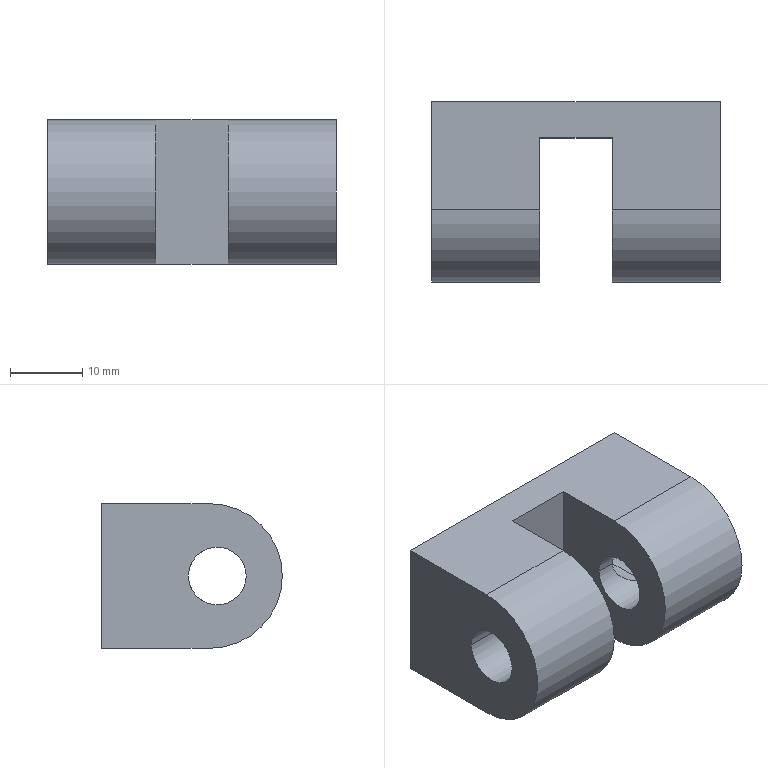Part | SolidWorks | features BaseBody 1 | 1 solid | 18 faces | box 40 x 25 x 20 mm | volume 12303 mm3 | cylinder 10 | plane 8 | commonest cylinder face diameters 6.8 x4 8 x4 20 x2
STEP:
#1=CARTESIAN_POINT('',(5.,-7.5,10.));
#2=VERTEX_POINT('',#1);
#3=CARTESIAN_POINT('',(5.,0.5,10.));
#4=VERTEX_POINT('',#3);
#5=CARTESIAN_POINT('',(5.,-3.5,10.));
#6=DIRECTION('',(1.,0.,0.));
#7=DIRECTION('',(0.,0.,-1.));
#8=AXIS2_PLACEMENT_3D('',#5,#6,#7);
#9=CIRCLE('',#8,4.);
#10=EDGE_CURVE('',#2,#4,#9,.T.);
#11=ORIENTED_EDGE('',*,*,#10,.F.);
#12=CARTESIAN_POINT('',(20.,-7.5,10.));
#13=VERTEX_POINT('',#12);
#14=CARTESIAN_POINT('',(-20.,-7.5,10.));
#15=DIRECTION('',(1.,0.,0.));
#16=VECTOR('',#15,1000.);
#17=LINE('',#14,#16);
#18=EDGE_CURVE('',#2,#13,#17,.T.);
#19=ORIENTED_EDGE('',*,*,#18,.T.);
#20=CARTESIAN_POINT('',(20.,0.5,10.));
#21=VERTEX_POINT('',#20);
#22=CARTESIAN_POINT('',(20.,-3.5,10.));
#23=DIRECTION('',(1.,0.,0.));
#24=DIRECTION('',(0.,1.,0.));
#25=AXIS2_PLACEMENT_3D('',#22,#23,#24);
#26=CIRCLE('',#25,4.);
#27=EDGE_CURVE('',#13,#21,#26,.T.);
#28=ORIENTED_EDGE('',*,*,#27,.T.);
#29=CARTESIAN_POINT('',(14.4,0.5,10.));
#30=VERTEX_POINT('',#29);
#31=CARTESIAN_POINT('',(-20.,0.5,10.));
#32=DIRECTION('',(1.,0.,0.));
#33=VECTOR('',#32,1000.);
#34=LINE('',#31,#33);
#35=EDGE_CURVE('',#30,#21,#34,.T.);
#36=ORIENTED_EDGE('',*,*,#35,.F.);
#37=CARTESIAN_POINT('',(11.,-1.393,6.6));
#38=VERTEX_POINT('',#37);
#39=CARTESIAN_POINT('',(11.,-1.393,6.6));
#40=CARTESIAN_POINT('',(11.242,-1.393,6.6));
#41=CARTESIAN_POINT('',(11.476,-1.35,6.626));
#42=CARTESIAN_POINT('',(11.927,-1.208,6.721));
#43=CARTESIAN_POINT('',(12.134,-1.113,6.788));
#44=CARTESIAN_POINT('',(12.529,-0.9021,6.956));
#45=CARTESIAN_POINT('',(12.715,-0.7863,7.057));
#46=CARTESIAN_POINT('',(13.06,-0.5558,7.287));
#47=CARTESIAN_POINT('',(13.221,-0.44,7.417));
#48=CARTESIAN_POINT('',(13.522,-0.2151,7.71));
#49=CARTESIAN_POINT('',(13.662,-0.1055,7.874));
#50=CARTESIAN_POINT('',(13.91,0.09224,8.229));
#51=CARTESIAN_POINT('',(14.019,0.1816,8.42));
#52=CARTESIAN_POINT('',(14.204,0.3341,8.838));
#53=CARTESIAN_POINT('',(14.275,0.3945,9.058));
#54=CARTESIAN_POINT('',(14.374,0.4777,9.518));
#55=CARTESIAN_POINT('',(14.4,0.5,9.759));
#56=CARTESIAN_POINT('',(14.4,0.5,10.));
#57=B_SPLINE_CURVE_WITH_KNOTS('',3,(#39,#40,#41,#42,#43,#44,#45,#46,#47,#48,#49,#50,#51,#52,#53,#54,#55,#56),.UNSPECIFIED.,.F.,.F.,(4,2,2,2,2,2,2,2,4),(0.,0.0007143,0.001429,0.002143,0.002857,0.003571,0.004286,0.005,0.005714),.UNSPECIFIED.);
#58=EDGE_CURVE('',#38,#30,#57,.T.);
#59=ORIENTED_EDGE('',*,*,#58,.F.);
#60=CARTESIAN_POINT('',(7.6,0.5,10.));
#61=VERTEX_POINT('',#60);
#62=CARTESIAN_POINT('',(7.6,0.5,10.));
#63=CARTESIAN_POINT('',(7.6,0.5,9.759));
#64=CARTESIAN_POINT('',(7.625,0.4783,9.523));
#65=CARTESIAN_POINT('',(7.723,0.396,9.064));
#66=CARTESIAN_POINT('',(7.796,0.3345,8.84));
#67=CARTESIAN_POINT('',(7.978,0.1841,8.426));
#68=CARTESIAN_POINT('',(8.088,0.09337,8.231));
#69=CARTESIAN_POINT('',(8.337,-0.1049,7.875));
#70=CARTESIAN_POINT('',(8.474,-0.2123,7.714));
#71=CARTESIAN_POINT('',(8.774,-0.4367,7.421));
#72=CARTESIAN_POINT('',(8.938,-0.5549,7.288));
#73=CARTESIAN_POINT('',(9.285,-0.786,7.057));
#74=CARTESIAN_POINT('',(9.467,-0.8998,6.957));
#75=CARTESIAN_POINT('',(9.861,-1.11,6.789));
#76=CARTESIAN_POINT('',(10.073,-1.208,6.721));
#77=CARTESIAN_POINT('',(10.519,-1.349,6.627));
#78=CARTESIAN_POINT('',(10.758,-1.393,6.6));
#79=CARTESIAN_POINT('',(11.,-1.393,6.6));
#80=B_SPLINE_CURVE_WITH_KNOTS('',3,(#62,#63,#64,#65,#66,#67,#68,#69,#70,#71,#72,#73,#74,#75,#76,#77,#78,#79),.UNSPECIFIED.,.F.,.F.,(4,2,2,2,2,2,2,2,4),(0.01715,0.01786,0.01858,0.01929,0.02001,0.02072,0.02144,0.02215,0.02287),.UNSPECIFIED.);
#81=EDGE_CURVE('',#61,#38,#80,.T.);
#82=ORIENTED_EDGE('',*,*,#81,.F.);
#83=CARTESIAN_POINT('',(-20.,0.5,10.));
#84=DIRECTION('',(1.,0.,0.));
#85=VECTOR('',#84,1000.);
#86=LINE('',#83,#85);
#87=EDGE_CURVE('',#4,#61,#86,.T.);
#88=ORIENTED_EDGE('',*,*,#87,.F.);
#89=EDGE_LOOP('',(#11,#19,#28,#36,#59,#82,#88));
#90=FACE_OUTER_BOUND('',#89,.T.);
#91=CARTESIAN_POINT('',(-20.,-3.5,10.));
#92=DIRECTION('',(1.,0.,0.));
#93=DIRECTION('',(0.,1.,0.));
#94=AXIS2_PLACEMENT_3D('',#91,#92,#93);
#95=CYLINDRICAL_SURFACE('',#94,4.);
#96=ADVANCED_FACE('',(#90),#95,.F.);
#97=CARTESIAN_POINT('',(-20.,-7.5,10.));
#98=VERTEX_POINT('',#97);
#99=CARTESIAN_POINT('',(-20.,0.5,10.));
#100=VERTEX_POINT('',#99);
#101=CARTESIAN_POINT('',(-20.,-3.5,10.));
#102=DIRECTION('',(1.,0.,0.));
#103=DIRECTION('',(0.,1.,0.));
#104=AXIS2_PLACEMENT_3D('',#101,#102,#103);
#105=CIRCLE('',#104,4.);
#106=EDGE_CURVE('',#98,#100,#105,.T.);
#107=ORIENTED_EDGE('',*,*,#106,.F.);
#108=CARTESIAN_POINT('',(-5.,-7.5,10.));
#109=VERTEX_POINT('',#108);
#110=CARTESIAN_POINT('',(-20.,-7.5,10.));
#111=DIRECTION('',(1.,0.,0.));
#112=VECTOR('',#111,1000.);
#113=LINE('',#110,#112);
#114=EDGE_CURVE('',#98,#109,#113,.T.);
#115=ORIENTED_EDGE('',*,*,#114,.T.);
#116=CARTESIAN_POINT('',(-5.,0.5,10.));
#117=VERTEX_POINT('',#116);
#118=CARTESIAN_POINT('',(-5.,-3.5,10.));
#119=DIRECTION('',(-1.,0.,0.));
#120=DIRECTION('',(0.,0.,1.));
#121=AXIS2_PLACEMENT_3D('',#118,#119,#120);
#122=CIRCLE('',#121,4.);
#123=EDGE_CURVE('',#117,#109,#122,.T.);
#124=ORIENTED_EDGE('',*,*,#123,.F.);
#125=CARTESIAN_POINT('',(-7.6,0.5,10.));
#126=VERTEX_POINT('',#125);
#127=CARTESIAN_POINT('',(-20.,0.5,10.));
#128=DIRECTION('',(1.,0.,0.));
#129=VECTOR('',#128,1000.);
#130=LINE('',#127,#129);
#131=EDGE_CURVE('',#126,#117,#130,.T.);
#132=ORIENTED_EDGE('',*,*,#131,.F.);
#133=CARTESIAN_POINT('',(-11.,-1.393,6.6));
#134=VERTEX_POINT('',#133);
#135=CARTESIAN_POINT('',(-11.,-1.393,6.6));
#136=CARTESIAN_POINT('',(-10.758,-1.393,6.6));
#137=CARTESIAN_POINT('',(-10.524,-1.35,6.626));
#138=CARTESIAN_POINT('',(-10.073,-1.208,6.721));
#139=CARTESIAN_POINT('',(-9.866,-1.113,6.788));
#140=CARTESIAN_POINT('',(-9.471,-0.9021,6.956));
#141=CARTESIAN_POINT('',(-9.285,-0.7863,7.057));
#142=CARTESIAN_POINT('',(-8.94,-0.5558,7.287));
#143=CARTESIAN_POINT('',(-8.779,-0.44,7.417));
#144=CARTESIAN_POINT('',(-8.478,-0.2151,7.71));
#145=CARTESIAN_POINT('',(-8.338,-0.1055,7.874));
#146=CARTESIAN_POINT('',(-8.09,0.09224,8.229));
#147=CARTESIAN_POINT('',(-7.981,0.1816,8.42));
#148=CARTESIAN_POINT('',(-7.796,0.3341,8.838));
#149=CARTESIAN_POINT('',(-7.725,0.3945,9.058));
#150=CARTESIAN_POINT('',(-7.626,0.4777,9.518));
#151=CARTESIAN_POINT('',(-7.6,0.5,9.759));
#152=CARTESIAN_POINT('',(-7.6,0.5,10.));
#153=B_SPLINE_CURVE_WITH_KNOTS('',3,(#135,#136,#137,#138,#139,#140,#141,#142,#143,#144,#145,#146,#147,#148,#149,#150,#151,#152),.UNSPECIFIED.,.F.,.F.,(4,2,2,2,2,2,2,2,4),(0.,0.0007143,0.001429,0.002143,0.002857,0.003571,0.004286,0.005,0.005714),.UNSPECIFIED.);
#154=EDGE_CURVE('',#134,#126,#153,.T.);
#155=ORIENTED_EDGE('',*,*,#154,.F.);
#156=CARTESIAN_POINT('',(-14.4,0.5,10.));
#157=VERTEX_POINT('',#156);
#158=CARTESIAN_POINT('',(-14.4,0.5,10.));
#159=CARTESIAN_POINT('',(-14.4,0.5,9.759));
#160=CARTESIAN_POINT('',(-14.375,0.4783,9.523));
#161=CARTESIAN_POINT('',(-14.277,0.396,9.064));
#162=CARTESIAN_POINT('',(-14.204,0.3345,8.84));
#163=CARTESIAN_POINT('',(-14.022,0.1841,8.426));
#164=CARTESIAN_POINT('',(-13.912,0.09337,8.231));
#165=CARTESIAN_POINT('',(-13.663,-0.1049,7.875));
#166=CARTESIAN_POINT('',(-13.526,-0.2123,7.714));
#167=CARTESIAN_POINT('',(-13.226,-0.4367,7.421));
#168=CARTESIAN_POINT('',(-13.062,-0.5549,7.288));
#169=CARTESIAN_POINT('',(-12.715,-0.786,7.057));
#170=CARTESIAN_POINT('',(-12.533,-0.8998,6.957));
#171=CARTESIAN_POINT('',(-12.139,-1.11,6.789));
#172=CARTESIAN_POINT('',(-11.927,-1.208,6.721));
#173=CARTESIAN_POINT('',(-11.481,-1.349,6.627));
#174=CARTESIAN_POINT('',(-11.242,-1.393,6.6));
#175=CARTESIAN_POINT('',(-11.,-1.393,6.6));
#176=B_SPLINE_CURVE_WITH_KNOTS('',3,(#158,#159,#160,#161,#162,#163,#164,#165,#166,#167,#168,#169,#170,#171,#172,#173,#174,#175),.UNSPECIFIED.,.F.,.F.,(4,2,2,2,2,2,2,2,4),(0.01715,0.01786,0.01858,0.01929,0.02001,0.02072,0.02144,0.02215,0.02287),.UNSPECIFIED.);
#177=EDGE_CURVE('',#157,#134,#176,.T.);
#178=ORIENTED_EDGE('',*,*,#177,.F.);
#179=CARTESIAN_POINT('',(-20.,0.5,10.));
#180=DIRECTION('',(1.,0.,0.));
#181=VECTOR('',#180,1000.);
#182=LINE('',#179,#181);
#183=EDGE_CURVE('',#100,#157,#182,.T.);
#184=ORIENTED_EDGE('',*,*,#183,.F.);
#185=EDGE_LOOP('',(#107,#115,#124,#132,#155,#178,#184));
#186=FACE_OUTER_BOUND('',#185,.T.);
#187=CARTESIAN_POINT('',(-20.,-3.5,10.));
#188=DIRECTION('',(1.,0.,0.));
#189=DIRECTION('',(0.,1.,0.));
#190=AXIS2_PLACEMENT_3D('',#187,#188,#189);
#191=CYLINDRICAL_SURFACE('',#190,4.);
#192=ADVANCED_FACE('',(#186),#191,.F.);
#193=CARTESIAN_POINT('',(-11.,-1.393,13.4));
#194=VERTEX_POINT('',#193);
#195=CARTESIAN_POINT('',(-11.,-1.393,13.4));
#196=CARTESIAN_POINT('',(-11.242,-1.393,13.4));
#197=CARTESIAN_POINT('',(-11.476,-1.35,13.374));
#198=CARTESIAN_POINT('',(-11.927,-1.208,13.279));
#199=CARTESIAN_POINT('',(-12.134,-1.113,13.212));
#200=CARTESIAN_POINT('',(-12.529,-0.9021,13.044));
#201=CARTESIAN_POINT('',(-12.715,-0.7863,12.943));
#202=CARTESIAN_POINT('',(-13.06,-0.5558,12.713));
#203=CARTESIAN_POINT('',(-13.221,-0.44,12.583));
#204=CARTESIAN_POINT('',(-13.522,-0.2151,12.29));
#205=CARTESIAN_POINT('',(-13.662,-0.1055,12.126));
#206=CARTESIAN_POINT('',(-13.91,0.09224,11.771));
#207=CARTESIAN_POINT('',(-14.019,0.1816,11.58));
#208=CARTESIAN_POINT('',(-14.204,0.3341,11.162));
#209=CARTESIAN_POINT('',(-14.275,0.3945,10.942));
#210=CARTESIAN_POINT('',(-14.374,0.4777,10.482));
#211=CARTESIAN_POINT('',(-14.4,0.5,10.241));
#212=CARTESIAN_POINT('',(-14.4,0.5,10.));
#213=B_SPLINE_CURVE_WITH_KNOTS('',3,(#195,#196,#197,#198,#199,#200,#201,#202,#203,#204,#205,#206,#207,#208,#209,#210,#211,#212),.UNSPECIFIED.,.F.,.F.,(4,2,2,2,2,2,2,2,4),(0.01143,0.01214,0.01286,0.01357,0.01429,0.015,0.01572,0.01643,0.01715),.UNSPECIFIED.);
#214=EDGE_CURVE('',#194,#157,#213,.T.);
#215=ORIENTED_EDGE('',*,*,#214,.T.);
#216=ORIENTED_EDGE('',*,*,#177,.T.);
#217=CARTESIAN_POINT('',(-11.,12.5,6.6));
#218=VERTEX_POINT('',#217);
#219=CARTESIAN_POINT('',(-11.,12.5,6.6));
#220=DIRECTION('',(0.,1.,0.));
#221=VECTOR('',#220,1000.);
#222=LINE('',#219,#221);
#223=EDGE_CURVE('',#134,#218,#222,.T.);
#224=ORIENTED_EDGE('',*,*,#223,.T.);
#225=CARTESIAN_POINT('',(-11.,12.5,13.4));
#226=VERTEX_POINT('',#225);
#227=CARTESIAN_POINT('',(-11.,12.5,10.));
#228=DIRECTION('',(0.,1.,0.));
#229=DIRECTION('',(0.,0.,1.));
#230=AXIS2_PLACEMENT_3D('',#227,#228,#229);
#231=CIRCLE('',#230,3.4);
#232=EDGE_CURVE('',#218,#226,#231,.T.);
#233=ORIENTED_EDGE('',*,*,#232,.T.);
#234=CARTESIAN_POINT('',(-11.,12.5,13.4));
#235=DIRECTION('',(0.,1.,0.));
#236=VECTOR('',#235,1000.);
#237=LINE('',#234,#236);
#238=EDGE_CURVE('',#194,#226,#237,.T.);
#239=ORIENTED_EDGE('',*,*,#238,.F.);
#240=EDGE_LOOP('',(#215,#216,#224,#233,#239));
#241=FACE_OUTER_BOUND('',#240,.T.);
#242=CARTESIAN_POINT('',(-11.,12.5,10.));
#243=DIRECTION('',(0.,1.,0.));
#244=DIRECTION('',(0.,0.,1.));
#245=AXIS2_PLACEMENT_3D('',#242,#243,#244);
#246=CYLINDRICAL_SURFACE('',#245,3.4);
#247=ADVANCED_FACE('',(#241),#246,.F.);
#248=CARTESIAN_POINT('',(11.,-1.393,13.4));
#249=VERTEX_POINT('',#248);
#250=CARTESIAN_POINT('',(11.,-1.393,13.4));
#251=CARTESIAN_POINT('',(10.758,-1.393,13.4));
#252=CARTESIAN_POINT('',(10.524,-1.35,13.374));
#253=CARTESIAN_POINT('',(10.073,-1.208,13.279));
#254=CARTESIAN_POINT('',(9.866,-1.113,13.212));
#255=CARTESIAN_POINT('',(9.471,-0.9021,13.044));
#256=CARTESIAN_POINT('',(9.285,-0.7863,12.943));
#257=CARTESIAN_POINT('',(8.94,-0.5558,12.713));
#258=CARTESIAN_POINT('',(8.779,-0.44,12.583));
#259=CARTESIAN_POINT('',(8.478,-0.2151,12.29));
#260=CARTESIAN_POINT('',(8.338,-0.1055,12.126));
#261=CARTESIAN_POINT('',(8.09,0.09224,11.771));
#262=CARTESIAN_POINT('',(7.981,0.1816,11.58));
#263=CARTESIAN_POINT('',(7.796,0.3341,11.162));
#264=CARTESIAN_POINT('',(7.725,0.3945,10.942));
#265=CARTESIAN_POINT('',(7.626,0.4777,10.482));
#266=CARTESIAN_POINT('',(7.6,0.5,10.241));
#267=CARTESIAN_POINT('',(7.6,0.5,10.));
#268=B_SPLINE_CURVE_WITH_KNOTS('',3,(#250,#251,#252,#253,#254,#255,#256,#257,#258,#259,#260,#261,#262,#263,#264,#265,#266,#267),.UNSPECIFIED.,.F.,.F.,(4,2,2,2,2,2,2,2,4),(0.01143,0.01214,0.01286,0.01357,0.01429,0.015,0.01572,0.01643,0.01715),.UNSPECIFIED.);
#269=EDGE_CURVE('',#249,#61,#268,.T.);
#270=ORIENTED_EDGE('',*,*,#269,.T.);
#271=ORIENTED_EDGE('',*,*,#81,.T.);
#272=CARTESIAN_POINT('',(11.,12.5,6.6));
#273=VERTEX_POINT('',#272);
#274=CARTESIAN_POINT('',(11.,12.5,6.6));
#275=DIRECTION('',(0.,1.,0.));
#276=VECTOR('',#275,1000.);
#277=LINE('',#274,#276);
#278=EDGE_CURVE('',#38,#273,#277,.T.);
#279=ORIENTED_EDGE('',*,*,#278,.T.);
#280=CARTESIAN_POINT('',(11.,12.5,13.4));
#281=VERTEX_POINT('',#280);
#282=CARTESIAN_POINT('',(11.,12.5,10.));
#283=DIRECTION('',(0.,1.,0.));
#284=DIRECTION('',(0.,0.,1.));
#285=AXIS2_PLACEMENT_3D('',#282,#283,#284);
#286=CIRCLE('',#285,3.4);
#287=EDGE_CURVE('',#273,#281,#286,.T.);
#288=ORIENTED_EDGE('',*,*,#287,.T.);
#289=CARTESIAN_POINT('',(11.,12.5,13.4));
#290=DIRECTION('',(0.,1.,0.));
#291=VECTOR('',#290,1000.);
#292=LINE('',#289,#291);
#293=EDGE_CURVE('',#249,#281,#292,.T.);
#294=ORIENTED_EDGE('',*,*,#293,.F.);
#295=EDGE_LOOP('',(#270,#271,#279,#288,#294));
#296=FACE_OUTER_BOUND('',#295,.T.);
#297=CARTESIAN_POINT('',(11.,12.5,10.));
#298=DIRECTION('',(0.,1.,0.));
#299=DIRECTION('',(0.,0.,1.));
#300=AXIS2_PLACEMENT_3D('',#297,#298,#299);
#301=CYLINDRICAL_SURFACE('',#300,3.4);
#302=ADVANCED_FACE('',(#296),#301,.F.);
#303=CARTESIAN_POINT('',(20.,-2.5,0.));
#304=VERTEX_POINT('',#303);
#305=CARTESIAN_POINT('',(5.,-2.5,0.));
#306=VERTEX_POINT('',#305);
#307=CARTESIAN_POINT('',(0.,-2.5,0.));
#308=DIRECTION('',(-1.,0.,0.));
#309=VECTOR('',#308,1000.);
#310=LINE('',#307,#309);
#311=EDGE_CURVE('',#304,#306,#310,.T.);
#312=ORIENTED_EDGE('',*,*,#311,.F.);
#313=CARTESIAN_POINT('',(20.,-2.5,20.));
#314=VERTEX_POINT('',#313);
#315=CARTESIAN_POINT('',(20.,-2.5,10.));
#316=DIRECTION('',(1.,0.,0.));
#317=DIRECTION('',(0.,-1.,0.));
#318=AXIS2_PLACEMENT_3D('',#315,#316,#317);
#319=CIRCLE('',#318,10.);
#320=EDGE_CURVE('',#314,#304,#319,.T.);
#321=ORIENTED_EDGE('',*,*,#320,.F.);
#322=CARTESIAN_POINT('',(5.,-2.5,20.));
#323=VERTEX_POINT('',#322);
#324=CARTESIAN_POINT('',(20.,-2.5,20.));
#325=DIRECTION('',(1.,0.,0.));
#326=VECTOR('',#325,1000.);
#327=LINE('',#324,#326);
#328=EDGE_CURVE('',#323,#314,#327,.T.);
#329=ORIENTED_EDGE('',*,*,#328,.F.);
#330=CARTESIAN_POINT('',(5.,-2.5,10.));
#331=DIRECTION('',(-1.,0.,0.));
#332=DIRECTION('',(0.,0.,-1.));
#333=AXIS2_PLACEMENT_3D('',#330,#331,#332);
#334=CIRCLE('',#333,10.);
#335=EDGE_CURVE('',#306,#323,#334,.T.);
#336=ORIENTED_EDGE('',*,*,#335,.F.);
#337=EDGE_LOOP('',(#312,#321,#329,#336));
#338=FACE_OUTER_BOUND('',#337,.T.);
#339=CARTESIAN_POINT('',(-20.,-2.5,10.));
#340=DIRECTION('',(1.,0.,0.));
#341=DIRECTION('',(0.,0.,-1.));
#342=AXIS2_PLACEMENT_3D('',#339,#340,#341);
#343=CYLINDRICAL_SURFACE('',#342,10.);
#344=ADVANCED_FACE('',(#338),#343,.T.);
#345=CARTESIAN_POINT('',(-5.,-2.5,0.));
#346=VERTEX_POINT('',#345);
#347=CARTESIAN_POINT('',(-20.,-2.5,0.));
#348=VERTEX_POINT('',#347);
#349=CARTESIAN_POINT('',(0.,-2.5,0.));
#350=DIRECTION('',(-1.,0.,0.));
#351=VECTOR('',#350,1000.);
#352=LINE('',#349,#351);
#353=EDGE_CURVE('',#346,#348,#352,.T.);
#354=ORIENTED_EDGE('',*,*,#353,.F.);
#355=CARTESIAN_POINT('',(-5.,-2.5,20.));
#356=VERTEX_POINT('',#355);
#357=CARTESIAN_POINT('',(-5.,-2.5,10.));
#358=DIRECTION('',(1.,0.,0.));
#359=DIRECTION('',(0.,0.,1.));
#360=AXIS2_PLACEMENT_3D('',#357,#358,#359);
#361=CIRCLE('',#360,10.);
#362=EDGE_CURVE('',#356,#346,#361,.T.);
#363=ORIENTED_EDGE('',*,*,#362,.F.);
#364=CARTESIAN_POINT('',(-20.,-2.5,20.));
#365=VERTEX_POINT('',#364);
#366=CARTESIAN_POINT('',(-5.,-2.5,20.));
#367=DIRECTION('',(1.,0.,0.));
#368=VECTOR('',#367,1000.);
#369=LINE('',#366,#368);
#370=EDGE_CURVE('',#365,#356,#369,.T.);
#371=ORIENTED_EDGE('',*,*,#370,.F.);
#372=CARTESIAN_POINT('',(-20.,-2.5,10.));
#373=DIRECTION('',(-1.,0.,0.));
#374=DIRECTION('',(0.,1.,0.));
#375=AXIS2_PLACEMENT_3D('',#372,#373,#374);
#376=CIRCLE('',#375,10.);
#377=EDGE_CURVE('',#348,#365,#376,.T.);
#378=ORIENTED_EDGE('',*,*,#377,.F.);
#379=EDGE_LOOP('',(#354,#363,#371,#378));
#380=FACE_OUTER_BOUND('',#379,.T.);
#381=CARTESIAN_POINT('',(-20.,-2.5,10.));
#382=DIRECTION('',(1.,0.,0.));
#383=DIRECTION('',(0.,0.,-1.));
#384=AXIS2_PLACEMENT_3D('',#381,#382,#383);
#385=CYLINDRICAL_SURFACE('',#384,10.);
#386=ADVANCED_FACE('',(#380),#385,.T.);
#387=CARTESIAN_POINT('',(5.,-3.5,10.));
#388=DIRECTION('',(1.,0.,0.));
#389=DIRECTION('',(0.,0.,-1.));
#390=AXIS2_PLACEMENT_3D('',#387,#388,#389);
#391=CIRCLE('',#390,4.);
#392=EDGE_CURVE('',#4,#2,#391,.T.);
#393=ORIENTED_EDGE('',*,*,#392,.T.);
#394=ORIENTED_EDGE('',*,*,#10,.T.);
#395=EDGE_LOOP('',(#393,#394));
#396=FACE_BOUND('',#395,.T.);
#397=ORIENTED_EDGE('',*,*,#335,.T.);
#398=CARTESIAN_POINT('',(5.,7.5,20.));
#399=VERTEX_POINT('',#398);
#400=CARTESIAN_POINT('',(5.,-12.5,20.));
#401=DIRECTION('',(0.,1.,0.));
#402=VECTOR('',#401,1000.);
#403=LINE('',#400,#402);
#404=EDGE_CURVE('',#323,#399,#403,.T.);
#405=ORIENTED_EDGE('',*,*,#404,.T.);
#406=CARTESIAN_POINT('',(5.,7.5,0.));
#407=VERTEX_POINT('',#406);
#408=CARTESIAN_POINT('',(5.,7.5,0.));
#409=DIRECTION('',(0.,0.,1.));
#410=VECTOR('',#409,1000.);
#411=LINE('',#408,#410);
#412=EDGE_CURVE('',#407,#399,#411,.T.);
#413=ORIENTED_EDGE('',*,*,#412,.F.);
#414=CARTESIAN_POINT('',(5.,-12.5,0.));
#415=DIRECTION('',(0.,1.,0.));
#416=VECTOR('',#415,1000.);
#417=LINE('',#414,#416);
#418=EDGE_CURVE('',#306,#407,#417,.T.);
#419=ORIENTED_EDGE('',*,*,#418,.F.);
#420=EDGE_LOOP('',(#397,#405,#413,#419));
#421=FACE_OUTER_BOUND('',#420,.T.);
#422=CARTESIAN_POINT('',(5.,-12.5,0.));
#423=DIRECTION('',(1.,0.,0.));
#424=DIRECTION('',(0.,1.,0.));
#425=AXIS2_PLACEMENT_3D('',#422,#423,#424);
#426=PLANE('',#425);
#427=ADVANCED_FACE('',(#396,#421),#426,.F.);
#428=CARTESIAN_POINT('',(-5.,7.5,20.));
#429=VERTEX_POINT('',#428);
#430=CARTESIAN_POINT('',(-5.,7.5,20.));
#431=DIRECTION('',(-1.,0.,0.));
#432=VECTOR('',#431,1000.);
#433=LINE('',#430,#432);
#434=EDGE_CURVE('',#399,#429,#433,.T.);
#435=ORIENTED_EDGE('',*,*,#434,.T.);
#436=CARTESIAN_POINT('',(-5.,7.5,0.));
#437=VERTEX_POINT('',#436);
#438=CARTESIAN_POINT('',(-5.,7.5,0.));
#439=DIRECTION('',(0.,0.,1.));
#440=VECTOR('',#439,1000.);
#441=LINE('',#438,#440);
#442=EDGE_CURVE('',#437,#429,#441,.T.);
#443=ORIENTED_EDGE('',*,*,#442,.F.);
#444=CARTESIAN_POINT('',(-5.,7.5,0.));
#445=DIRECTION('',(-1.,0.,0.));
#446=VECTOR('',#445,1000.);
#447=LINE('',#444,#446);
#448=EDGE_CURVE('',#407,#437,#447,.T.);
#449=ORIENTED_EDGE('',*,*,#448,.F.);
#450=ORIENTED_EDGE('',*,*,#412,.T.);
#451=EDGE_LOOP('',(#435,#443,#449,#450));
#452=FACE_OUTER_BOUND('',#451,.T.);
#453=CARTESIAN_POINT('',(-5.,7.5,0.));
#454=DIRECTION('',(0.,1.,0.));
#455=DIRECTION('',(1.,0.,0.));
#456=AXIS2_PLACEMENT_3D('',#453,#454,#455);
#457=PLANE('',#456);
#458=ADVANCED_FACE('',(#452),#457,.F.);
#459=ORIENTED_EDGE('',*,*,#123,.T.);
#460=CARTESIAN_POINT('',(-5.,-3.5,10.));
#461=DIRECTION('',(-1.,0.,0.));
#462=DIRECTION('',(0.,0.,1.));
#463=AXIS2_PLACEMENT_3D('',#460,#461,#462);
#464=CIRCLE('',#463,4.);
#465=EDGE_CURVE('',#109,#117,#464,.T.);
#466=ORIENTED_EDGE('',*,*,#465,.T.);
#467=EDGE_LOOP('',(#459,#466));
#468=FACE_BOUND('',#467,.T.);
#469=CARTESIAN_POINT('',(-5.,-12.5,20.));
#470=DIRECTION('',(0.,-1.,0.));
#471=VECTOR('',#470,1000.);
#472=LINE('',#469,#471);
#473=EDGE_CURVE('',#429,#356,#472,.T.);
#474=ORIENTED_EDGE('',*,*,#473,.T.);
#475=ORIENTED_EDGE('',*,*,#362,.T.);
#476=CARTESIAN_POINT('',(-5.,-12.5,0.));
#477=DIRECTION('',(0.,-1.,0.));
#478=VECTOR('',#477,1000.);
#479=LINE('',#476,#478);
#480=EDGE_CURVE('',#437,#346,#479,.T.);
#481=ORIENTED_EDGE('',*,*,#480,.F.);
#482=ORIENTED_EDGE('',*,*,#442,.T.);
#483=EDGE_LOOP('',(#474,#475,#481,#482));
#484=FACE_OUTER_BOUND('',#483,.T.);
#485=CARTESIAN_POINT('',(-5.,-12.5,0.));
#486=DIRECTION('',(-1.,0.,0.));
#487=DIRECTION('',(0.,0.,1.));
#488=AXIS2_PLACEMENT_3D('',#485,#486,#487);
#489=PLANE('',#488);
#490=ADVANCED_FACE('',(#468,#484),#489,.F.);
#491=ORIENTED_EDGE('',*,*,#480,.T.);
#492=ORIENTED_EDGE('',*,*,#353,.T.);
#493=CARTESIAN_POINT('',(-20.,12.5,0.));
#494=VERTEX_POINT('',#493);
#495=CARTESIAN_POINT('',(-20.,12.5,0.));
#496=DIRECTION('',(0.,-1.,0.));
#497=VECTOR('',#496,1000.);
#498=LINE('',#495,#497);
#499=EDGE_CURVE('',#494,#348,#498,.T.);
#500=ORIENTED_EDGE('',*,*,#499,.F.);
#501=CARTESIAN_POINT('',(20.,12.5,0.));
#502=VERTEX_POINT('',#501);
#503=CARTESIAN_POINT('',(-20.,12.5,0.));
#504=DIRECTION('',(-1.,0.,0.));
#505=VECTOR('',#504,1000.);
#506=LINE('',#503,#505);
#507=EDGE_CURVE('',#502,#494,#506,.T.);
#508=ORIENTED_EDGE('',*,*,#507,.F.);
#509=CARTESIAN_POINT('',(20.,12.5,0.));
#510=DIRECTION('',(0.,1.,0.));
#511=VECTOR('',#510,1000.);
#512=LINE('',#509,#511);
#513=EDGE_CURVE('',#304,#502,#512,.T.);
#514=ORIENTED_EDGE('',*,*,#513,.F.);
#515=ORIENTED_EDGE('',*,*,#311,.T.);
#516=ORIENTED_EDGE('',*,*,#418,.T.);
#517=ORIENTED_EDGE('',*,*,#448,.T.);
#518=EDGE_LOOP('',(#491,#492,#500,#508,#514,#515,#516,#517));
#519=FACE_OUTER_BOUND('',#518,.T.);
#520=CARTESIAN_POINT('',(0.,0.,0.));
#521=DIRECTION('',(0.,0.,1.));
#522=DIRECTION('',(1.,0.,0.));
#523=AXIS2_PLACEMENT_3D('',#520,#521,#522);
#524=PLANE('',#523);
#525=ADVANCED_FACE('',(#519),#524,.F.);
#526=CARTESIAN_POINT('',(-20.,12.5,20.));
#527=VERTEX_POINT('',#526);
#528=CARTESIAN_POINT('',(-20.,12.5,20.));
#529=DIRECTION('',(0.,-1.,0.));
#530=VECTOR('',#529,1000.);
#531=LINE('',#528,#530);
#532=EDGE_CURVE('',#527,#365,#531,.T.);
#533=ORIENTED_EDGE('',*,*,#532,.T.);
#534=ORIENTED_EDGE('',*,*,#370,.T.);
#535=ORIENTED_EDGE('',*,*,#473,.F.);
#536=ORIENTED_EDGE('',*,*,#434,.F.);
#537=ORIENTED_EDGE('',*,*,#404,.F.);
#538=ORIENTED_EDGE('',*,*,#328,.T.);
#539=CARTESIAN_POINT('',(20.,12.5,20.));
#540=VERTEX_POINT('',#539);
#541=CARTESIAN_POINT('',(20.,12.5,20.));
#542=DIRECTION('',(0.,1.,0.));
#543=VECTOR('',#542,1000.);
#544=LINE('',#541,#543);
#545=EDGE_CURVE('',#314,#540,#544,.T.);
#546=ORIENTED_EDGE('',*,*,#545,.T.);
#547=CARTESIAN_POINT('',(-20.,12.5,20.));
#548=DIRECTION('',(-1.,0.,0.));
#549=VECTOR('',#548,1000.);
#550=LINE('',#547,#549);
#551=EDGE_CURVE('',#540,#527,#550,.T.);
#552=ORIENTED_EDGE('',*,*,#551,.T.);
#553=EDGE_LOOP('',(#533,#534,#535,#536,#537,#538,#546,#552));
#554=FACE_OUTER_BOUND('',#553,.T.);
#555=CARTESIAN_POINT('',(0.,0.,20.));
#556=DIRECTION('',(0.,0.,1.));
#557=DIRECTION('',(1.,0.,0.));
#558=AXIS2_PLACEMENT_3D('',#555,#556,#557);
#559=PLANE('',#558);
#560=ADVANCED_FACE('',(#554),#559,.T.);
#561=CARTESIAN_POINT('',(-20.,-3.5,10.));
#562=DIRECTION('',(1.,0.,0.));
#563=DIRECTION('',(0.,1.,0.));
#564=AXIS2_PLACEMENT_3D('',#561,#562,#563);
#565=CIRCLE('',#564,4.);
#566=EDGE_CURVE('',#100,#98,#565,.T.);
#567=ORIENTED_EDGE('',*,*,#566,.T.);
#568=ORIENTED_EDGE('',*,*,#106,.T.);
#569=EDGE_LOOP('',(#567,#568));
#570=FACE_BOUND('',#569,.T.);
#571=ORIENTED_EDGE('',*,*,#377,.T.);
#572=ORIENTED_EDGE('',*,*,#532,.F.);
#573=CARTESIAN_POINT('',(-20.,12.5,20.));
#574=DIRECTION('',(0.,0.,-1.));
#575=VECTOR('',#574,1000.);
#576=LINE('',#573,#575);
#577=EDGE_CURVE('',#527,#494,#576,.T.);
#578=ORIENTED_EDGE('',*,*,#577,.T.);
#579=ORIENTED_EDGE('',*,*,#499,.T.);
#580=EDGE_LOOP('',(#571,#572,#578,#579));
#581=FACE_OUTER_BOUND('',#580,.T.);
#582=CARTESIAN_POINT('',(-20.,12.5,20.));
#583=DIRECTION('',(1.,0.,0.));
#584=DIRECTION('',(0.,1.,0.));
#585=AXIS2_PLACEMENT_3D('',#582,#583,#584);
#586=PLANE('',#585);
#587=ADVANCED_FACE('',(#570,#581),#586,.F.);
#588=CARTESIAN_POINT('',(11.,12.5,10.));
#589=DIRECTION('',(0.,1.,0.));
#590=DIRECTION('',(0.,0.,1.));
#591=AXIS2_PLACEMENT_3D('',#588,#589,#590);
#592=CIRCLE('',#591,3.4);
#593=EDGE_CURVE('',#281,#273,#592,.T.);
#594=ORIENTED_EDGE('',*,*,#593,.F.);
#595=ORIENTED_EDGE('',*,*,#287,.F.);
#596=EDGE_LOOP('',(#594,#595));
#597=FACE_BOUND('',#596,.T.);
#598=CARTESIAN_POINT('',(-11.,12.5,10.));
#599=DIRECTION('',(0.,1.,0.));
#600=DIRECTION('',(0.,0.,1.));
#601=AXIS2_PLACEMENT_3D('',#598,#599,#600);
#602=CIRCLE('',#601,3.4);
#603=EDGE_CURVE('',#226,#218,#602,.T.);
#604=ORIENTED_EDGE('',*,*,#603,.F.);
#605=ORIENTED_EDGE('',*,*,#232,.F.);
#606=EDGE_LOOP('',(#604,#605));
#607=FACE_BOUND('',#606,.T.);
#608=ORIENTED_EDGE('',*,*,#507,.T.);
#609=ORIENTED_EDGE('',*,*,#577,.F.);
#610=ORIENTED_EDGE('',*,*,#551,.F.);
#611=CARTESIAN_POINT('',(20.,12.5,20.));
#612=DIRECTION('',(0.,0.,-1.));
#613=VECTOR('',#612,1000.);
#614=LINE('',#611,#613);
#615=EDGE_CURVE('',#540,#502,#614,.T.);
#616=ORIENTED_EDGE('',*,*,#615,.T.);
#617=EDGE_LOOP('',(#608,#609,#610,#616));
#618=FACE_OUTER_BOUND('',#617,.T.);
#619=CARTESIAN_POINT('',(-20.,12.5,20.));
#620=DIRECTION('',(0.,-1.,0.));
#621=DIRECTION('',(0.,0.,-1.));
#622=AXIS2_PLACEMENT_3D('',#619,#620,#621);
#623=PLANE('',#622);
#624=ADVANCED_FACE('',(#597,#607,#618),#623,.F.);
#625=CARTESIAN_POINT('',(20.,-3.5,10.));
#626=DIRECTION('',(1.,0.,0.));
#627=DIRECTION('',(0.,1.,0.));
#628=AXIS2_PLACEMENT_3D('',#625,#626,#627);
#629=CIRCLE('',#628,4.);
#630=EDGE_CURVE('',#21,#13,#629,.T.);
#631=ORIENTED_EDGE('',*,*,#630,.F.);
#632=ORIENTED_EDGE('',*,*,#27,.F.);
#633=EDGE_LOOP('',(#631,#632));
#634=FACE_BOUND('',#633,.T.);
#635=ORIENTED_EDGE('',*,*,#545,.F.);
#636=ORIENTED_EDGE('',*,*,#320,.T.);
#637=ORIENTED_EDGE('',*,*,#513,.T.);
#638=ORIENTED_EDGE('',*,*,#615,.F.);
#639=EDGE_LOOP('',(#635,#636,#637,#638));
#640=FACE_OUTER_BOUND('',#639,.T.);
#641=CARTESIAN_POINT('',(20.,12.5,20.));
#642=DIRECTION('',(-1.,0.,0.));
#643=DIRECTION('',(0.,1.,0.));
#644=AXIS2_PLACEMENT_3D('',#641,#642,#643);
#645=PLANE('',#644);
#646=ADVANCED_FACE('',(#634,#640),#645,.F.);
#647=ORIENTED_EDGE('',*,*,#278,.F.);
#648=ORIENTED_EDGE('',*,*,#58,.T.);
#649=CARTESIAN_POINT('',(14.4,0.5,10.));
#650=CARTESIAN_POINT('',(14.4,0.5,10.241));
#651=CARTESIAN_POINT('',(14.375,0.4783,10.477));
#652=CARTESIAN_POINT('',(14.277,0.396,10.936));
#653=CARTESIAN_POINT('',(14.204,0.3345,11.16));
#654=CARTESIAN_POINT('',(14.022,0.1841,11.574));
#655=CARTESIAN_POINT('',(13.912,0.09337,11.769));
#656=CARTESIAN_POINT('',(13.663,-0.1049,12.125));
#657=CARTESIAN_POINT('',(13.526,-0.2123,12.286));
#658=CARTESIAN_POINT('',(13.226,-0.4367,12.579));
#659=CARTESIAN_POINT('',(13.062,-0.5549,12.712));
#660=CARTESIAN_POINT('',(12.715,-0.786,12.943));
#661=CARTESIAN_POINT('',(12.533,-0.8998,13.043));
#662=CARTESIAN_POINT('',(12.139,-1.11,13.211));
#663=CARTESIAN_POINT('',(11.927,-1.208,13.279));
#664=CARTESIAN_POINT('',(11.481,-1.349,13.373));
#665=CARTESIAN_POINT('',(11.242,-1.393,13.4));
#666=CARTESIAN_POINT('',(11.,-1.393,13.4));
#667=B_SPLINE_CURVE_WITH_KNOTS('',3,(#649,#650,#651,#652,#653,#654,#655,#656,#657,#658,#659,#660,#661,#662,#663,#664,#665,#666),.UNSPECIFIED.,.F.,.F.,(4,2,2,2,2,2,2,2,4),(0.005714,0.006428,0.007143,0.007857,0.008571,0.009286,0.01,0.01071,0.01143),.UNSPECIFIED.);
#668=EDGE_CURVE('',#30,#249,#667,.T.);
#669=ORIENTED_EDGE('',*,*,#668,.T.);
#670=ORIENTED_EDGE('',*,*,#293,.T.);
#671=ORIENTED_EDGE('',*,*,#593,.T.);
#672=EDGE_LOOP('',(#647,#648,#669,#670,#671));
#673=FACE_OUTER_BOUND('',#672,.T.);
#674=CARTESIAN_POINT('',(11.,12.5,10.));
#675=DIRECTION('',(0.,1.,0.));
#676=DIRECTION('',(0.,0.,1.));
#677=AXIS2_PLACEMENT_3D('',#674,#675,#676);
#678=CYLINDRICAL_SURFACE('',#677,3.4);
#679=ADVANCED_FACE('',(#673),#678,.F.);
#680=ORIENTED_EDGE('',*,*,#223,.F.);
#681=ORIENTED_EDGE('',*,*,#154,.T.);
#682=CARTESIAN_POINT('',(-7.6,0.5,10.));
#683=CARTESIAN_POINT('',(-7.6,0.5,10.241));
#684=CARTESIAN_POINT('',(-7.625,0.4783,10.477));
#685=CARTESIAN_POINT('',(-7.723,0.396,10.936));
#686=CARTESIAN_POINT('',(-7.796,0.3345,11.16));
#687=CARTESIAN_POINT('',(-7.978,0.1841,11.574));
#688=CARTESIAN_POINT('',(-8.088,0.09337,11.769));
#689=CARTESIAN_POINT('',(-8.337,-0.1049,12.125));
#690=CARTESIAN_POINT('',(-8.474,-0.2123,12.286));
#691=CARTESIAN_POINT('',(-8.774,-0.4367,12.579));
#692=CARTESIAN_POINT('',(-8.938,-0.5549,12.712));
#693=CARTESIAN_POINT('',(-9.285,-0.786,12.943));
#694=CARTESIAN_POINT('',(-9.467,-0.8998,13.043));
#695=CARTESIAN_POINT('',(-9.861,-1.11,13.211));
#696=CARTESIAN_POINT('',(-10.073,-1.208,13.279));
#697=CARTESIAN_POINT('',(-10.519,-1.349,13.373));
#698=CARTESIAN_POINT('',(-10.758,-1.393,13.4));
#699=CARTESIAN_POINT('',(-11.,-1.393,13.4));
#700=B_SPLINE_CURVE_WITH_KNOTS('',3,(#682,#683,#684,#685,#686,#687,#688,#689,#690,#691,#692,#693,#694,#695,#696,#697,#698,#699),.UNSPECIFIED.,.F.,.F.,(4,2,2,2,2,2,2,2,4),(0.005714,0.006428,0.007143,0.007857,0.008571,0.009286,0.01,0.01071,0.01143),.UNSPECIFIED.);
#701=EDGE_CURVE('',#126,#194,#700,.T.);
#702=ORIENTED_EDGE('',*,*,#701,.T.);
#703=ORIENTED_EDGE('',*,*,#238,.T.);
#704=ORIENTED_EDGE('',*,*,#603,.T.);
#705=EDGE_LOOP('',(#680,#681,#702,#703,#704));
#706=FACE_OUTER_BOUND('',#705,.T.);
#707=CARTESIAN_POINT('',(-11.,12.5,10.));
#708=DIRECTION('',(0.,1.,0.));
#709=DIRECTION('',(0.,0.,1.));
#710=AXIS2_PLACEMENT_3D('',#707,#708,#709);
#711=CYLINDRICAL_SURFACE('',#710,3.4);
#712=ADVANCED_FACE('',(#706),#711,.F.);
#713=ORIENTED_EDGE('',*,*,#114,.F.);
#714=ORIENTED_EDGE('',*,*,#566,.F.);
#715=ORIENTED_EDGE('',*,*,#183,.T.);
#716=ORIENTED_EDGE('',*,*,#214,.F.);
#717=ORIENTED_EDGE('',*,*,#701,.F.);
#718=ORIENTED_EDGE('',*,*,#131,.T.);
#719=ORIENTED_EDGE('',*,*,#465,.F.);
#720=EDGE_LOOP('',(#713,#714,#715,#716,#717,#718,#719));
#721=FACE_OUTER_BOUND('',#720,.T.);
#722=CARTESIAN_POINT('',(-20.,-3.5,10.));
#723=DIRECTION('',(1.,0.,0.));
#724=DIRECTION('',(0.,1.,0.));
#725=AXIS2_PLACEMENT_3D('',#722,#723,#724);
#726=CYLINDRICAL_SURFACE('',#725,4.);
#727=ADVANCED_FACE('',(#721),#726,.F.);
#728=ORIENTED_EDGE('',*,*,#18,.F.);
#729=ORIENTED_EDGE('',*,*,#392,.F.);
#730=ORIENTED_EDGE('',*,*,#87,.T.);
#731=ORIENTED_EDGE('',*,*,#269,.F.);
#732=ORIENTED_EDGE('',*,*,#668,.F.);
#733=ORIENTED_EDGE('',*,*,#35,.T.);
#734=ORIENTED_EDGE('',*,*,#630,.T.);
#735=EDGE_LOOP('',(#728,#729,#730,#731,#732,#733,#734));
#736=FACE_OUTER_BOUND('',#735,.T.);
#737=CARTESIAN_POINT('',(-20.,-3.5,10.));
#738=DIRECTION('',(1.,0.,0.));
#739=DIRECTION('',(0.,1.,0.));
#740=AXIS2_PLACEMENT_3D('',#737,#738,#739);
#741=CYLINDRICAL_SURFACE('',#740,4.);
#742=ADVANCED_FACE('',(#736),#741,.F.);
#743=CLOSED_SHELL('',(#96,#192,#247,#302,#344,#386,#427,#458,#490,#525,#560,#587,#624,#646,#679,#712,#727,#742));
#744=MANIFOLD_SOLID_BREP('',#743);
#745=CARTESIAN_POINT('',(0.,0.,0.));
#746=DIRECTION('',(0.,0.,1.));
#747=DIRECTION('',(1.,0.,0.));
#748=AXIS2_PLACEMENT_3D('',#745,#746,#747);
#749=(LENGTH_UNIT()NAMED_UNIT(*)SI_UNIT(.MILLI.,.METRE.));
#750=UNCERTAINTY_MEASURE_WITH_UNIT(LENGTH_MEASURE(0.00001),#749,'','');
#751=(NAMED_UNIT(*)PLANE_ANGLE_UNIT()SI_UNIT($,.RADIAN.));
#752=(NAMED_UNIT(*)SI_UNIT($,.STERADIAN.)SOLID_ANGLE_UNIT());
#753=(GEOMETRIC_REPRESENTATION_CONTEXT(3)GLOBAL_UNCERTAINTY_ASSIGNED_CONTEXT((#750))GLOBAL_UNIT_ASSIGNED_CONTEXT((#749,#751,#752))REPRESENTATION_CONTEXT('',''));
#754=ADVANCED_BREP_SHAPE_REPRESENTATION('',(#744,#748),#753);